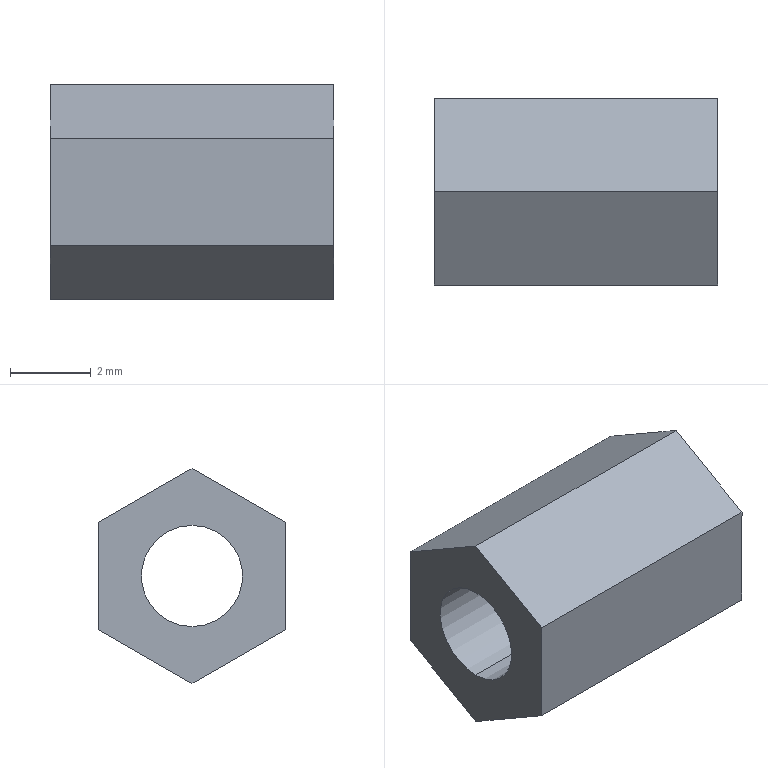Part | SolidWorks | features Extrusion 1, HoleWzd 1 | 1 solid | 10 faces | box 7 x 4.6 x 5.312 mm | volume 93.915 mm3 | plane 8 | cylinder 2 | commonest cylinder face diameters 2.5 x2
STEP:
#1=CARTESIAN_POINT('',(0.,0.,1.25));
#2=VERTEX_POINT('',#1);
#3=CARTESIAN_POINT('',(0.,0.,-1.25));
#4=VERTEX_POINT('',#3);
#5=CARTESIAN_POINT('',(0.,0.,0.));
#6=DIRECTION('',(1.,0.,0.));
#7=DIRECTION('',(0.,0.,-1.));
#8=AXIS2_PLACEMENT_3D('',#5,#6,#7);
#9=CIRCLE('',#8,1.25);
#10=EDGE_CURVE('',#2,#4,#9,.T.);
#11=ORIENTED_EDGE('',*,*,#10,.F.);
#12=CARTESIAN_POINT('',(7.,0.,1.25));
#13=VERTEX_POINT('',#12);
#14=CARTESIAN_POINT('',(7.,0.,1.25));
#15=DIRECTION('',(1.,0.,0.));
#16=VECTOR('',#15,1000.);
#17=LINE('',#14,#16);
#18=EDGE_CURVE('',#2,#13,#17,.T.);
#19=ORIENTED_EDGE('',*,*,#18,.T.);
#20=CARTESIAN_POINT('',(7.,0.,-1.25));
#21=VERTEX_POINT('',#20);
#22=CARTESIAN_POINT('',(7.,0.,0.));
#23=DIRECTION('',(1.,0.,0.));
#24=DIRECTION('',(0.,0.,-1.));
#25=AXIS2_PLACEMENT_3D('',#22,#23,#24);
#26=CIRCLE('',#25,1.25);
#27=EDGE_CURVE('',#13,#21,#26,.T.);
#28=ORIENTED_EDGE('',*,*,#27,.T.);
#29=CARTESIAN_POINT('',(7.,0.,-1.25));
#30=DIRECTION('',(1.,0.,0.));
#31=VECTOR('',#30,1000.);
#32=LINE('',#29,#31);
#33=EDGE_CURVE('',#4,#21,#32,.T.);
#34=ORIENTED_EDGE('',*,*,#33,.F.);
#35=EDGE_LOOP('',(#11,#19,#28,#34));
#36=FACE_OUTER_BOUND('',#35,.T.);
#37=CARTESIAN_POINT('',(7.,0.,0.));
#38=DIRECTION('',(1.,0.,0.));
#39=DIRECTION('',(0.,0.,-1.));
#40=AXIS2_PLACEMENT_3D('',#37,#38,#39);
#41=CYLINDRICAL_SURFACE('',#40,1.25);
#42=ADVANCED_FACE('',(#36),#41,.F.);
#43=CARTESIAN_POINT('',(0.,-2.3,-1.328));
#44=VERTEX_POINT('',#43);
#45=CARTESIAN_POINT('',(0.,0.,-2.656));
#46=VERTEX_POINT('',#45);
#47=CARTESIAN_POINT('',(0.,-2.3,-1.328));
#48=DIRECTION('',(0.,0.866,-0.5));
#49=VECTOR('',#48,1000.);
#50=LINE('',#47,#49);
#51=EDGE_CURVE('',#44,#46,#50,.T.);
#52=ORIENTED_EDGE('',*,*,#51,.T.);
#53=CARTESIAN_POINT('',(7.,0.,-2.656));
#54=VERTEX_POINT('',#53);
#55=CARTESIAN_POINT('',(7.,0.,-2.656));
#56=DIRECTION('',(-1.,0.,0.));
#57=VECTOR('',#56,1000.);
#58=LINE('',#55,#57);
#59=EDGE_CURVE('',#54,#46,#58,.T.);
#60=ORIENTED_EDGE('',*,*,#59,.F.);
#61=CARTESIAN_POINT('',(7.,-2.3,-1.328));
#62=VERTEX_POINT('',#61);
#63=CARTESIAN_POINT('',(7.,-2.3,-1.328));
#64=DIRECTION('',(0.,0.866,-0.5));
#65=VECTOR('',#64,1000.);
#66=LINE('',#63,#65);
#67=EDGE_CURVE('',#62,#54,#66,.T.);
#68=ORIENTED_EDGE('',*,*,#67,.F.);
#69=CARTESIAN_POINT('',(7.,-2.3,-1.328));
#70=DIRECTION('',(-1.,0.,0.));
#71=VECTOR('',#70,1000.);
#72=LINE('',#69,#71);
#73=EDGE_CURVE('',#62,#44,#72,.T.);
#74=ORIENTED_EDGE('',*,*,#73,.T.);
#75=EDGE_LOOP('',(#52,#60,#68,#74));
#76=FACE_OUTER_BOUND('',#75,.T.);
#77=CARTESIAN_POINT('',(7.,-2.3,-1.328));
#78=DIRECTION('',(0.,0.5,0.866));
#79=DIRECTION('',(0.,-0.866,0.5));
#80=AXIS2_PLACEMENT_3D('',#77,#78,#79);
#81=PLANE('',#80);
#82=ADVANCED_FACE('',(#76),#81,.F.);
#83=CARTESIAN_POINT('',(0.,2.3,-1.328));
#84=VERTEX_POINT('',#83);
#85=CARTESIAN_POINT('',(0.,0.,-2.656));
#86=DIRECTION('',(0.,0.866,0.5));
#87=VECTOR('',#86,1000.);
#88=LINE('',#85,#87);
#89=EDGE_CURVE('',#46,#84,#88,.T.);
#90=ORIENTED_EDGE('',*,*,#89,.T.);
#91=CARTESIAN_POINT('',(7.,2.3,-1.328));
#92=VERTEX_POINT('',#91);
#93=CARTESIAN_POINT('',(7.,2.3,-1.328));
#94=DIRECTION('',(-1.,0.,0.));
#95=VECTOR('',#94,1000.);
#96=LINE('',#93,#95);
#97=EDGE_CURVE('',#92,#84,#96,.T.);
#98=ORIENTED_EDGE('',*,*,#97,.F.);
#99=CARTESIAN_POINT('',(7.,0.,-2.656));
#100=DIRECTION('',(0.,0.866,0.5));
#101=VECTOR('',#100,1000.);
#102=LINE('',#99,#101);
#103=EDGE_CURVE('',#54,#92,#102,.T.);
#104=ORIENTED_EDGE('',*,*,#103,.F.);
#105=ORIENTED_EDGE('',*,*,#59,.T.);
#106=EDGE_LOOP('',(#90,#98,#104,#105));
#107=FACE_OUTER_BOUND('',#106,.T.);
#108=CARTESIAN_POINT('',(7.,0.,-2.656));
#109=DIRECTION('',(0.,-0.5,0.866));
#110=DIRECTION('',(0.,-0.866,-0.5));
#111=AXIS2_PLACEMENT_3D('',#108,#109,#110);
#112=PLANE('',#111);
#113=ADVANCED_FACE('',(#107),#112,.F.);
#114=CARTESIAN_POINT('',(0.,2.3,1.328));
#115=VERTEX_POINT('',#114);
#116=CARTESIAN_POINT('',(0.,2.3,-1.328));
#117=DIRECTION('',(0.,0.,1.));
#118=VECTOR('',#117,1000.);
#119=LINE('',#116,#118);
#120=EDGE_CURVE('',#84,#115,#119,.T.);
#121=ORIENTED_EDGE('',*,*,#120,.T.);
#122=CARTESIAN_POINT('',(7.,2.3,1.328));
#123=VERTEX_POINT('',#122);
#124=CARTESIAN_POINT('',(7.,2.3,1.328));
#125=DIRECTION('',(-1.,0.,0.));
#126=VECTOR('',#125,1000.);
#127=LINE('',#124,#126);
#128=EDGE_CURVE('',#123,#115,#127,.T.);
#129=ORIENTED_EDGE('',*,*,#128,.F.);
#130=CARTESIAN_POINT('',(7.,2.3,-1.328));
#131=DIRECTION('',(0.,0.,1.));
#132=VECTOR('',#131,1000.);
#133=LINE('',#130,#132);
#134=EDGE_CURVE('',#92,#123,#133,.T.);
#135=ORIENTED_EDGE('',*,*,#134,.F.);
#136=ORIENTED_EDGE('',*,*,#97,.T.);
#137=EDGE_LOOP('',(#121,#129,#135,#136));
#138=FACE_OUTER_BOUND('',#137,.T.);
#139=CARTESIAN_POINT('',(7.,2.3,-1.328));
#140=DIRECTION('',(0.,-1.,0.));
#141=DIRECTION('',(0.,0.,-1.));
#142=AXIS2_PLACEMENT_3D('',#139,#140,#141);
#143=PLANE('',#142);
#144=ADVANCED_FACE('',(#138),#143,.F.);
#145=CARTESIAN_POINT('',(0.,0.,2.656));
#146=VERTEX_POINT('',#145);
#147=CARTESIAN_POINT('',(0.,2.3,1.328));
#148=DIRECTION('',(0.,-0.866,0.5));
#149=VECTOR('',#148,1000.);
#150=LINE('',#147,#149);
#151=EDGE_CURVE('',#115,#146,#150,.T.);
#152=ORIENTED_EDGE('',*,*,#151,.T.);
#153=CARTESIAN_POINT('',(7.,0.,2.656));
#154=VERTEX_POINT('',#153);
#155=CARTESIAN_POINT('',(7.,0.,2.656));
#156=DIRECTION('',(-1.,0.,0.));
#157=VECTOR('',#156,1000.);
#158=LINE('',#155,#157);
#159=EDGE_CURVE('',#154,#146,#158,.T.);
#160=ORIENTED_EDGE('',*,*,#159,.F.);
#161=CARTESIAN_POINT('',(7.,2.3,1.328));
#162=DIRECTION('',(0.,-0.866,0.5));
#163=VECTOR('',#162,1000.);
#164=LINE('',#161,#163);
#165=EDGE_CURVE('',#123,#154,#164,.T.);
#166=ORIENTED_EDGE('',*,*,#165,.F.);
#167=ORIENTED_EDGE('',*,*,#128,.T.);
#168=EDGE_LOOP('',(#152,#160,#166,#167));
#169=FACE_OUTER_BOUND('',#168,.T.);
#170=CARTESIAN_POINT('',(7.,2.3,1.328));
#171=DIRECTION('',(0.,-0.5,-0.866));
#172=DIRECTION('',(0.,0.866,-0.5));
#173=AXIS2_PLACEMENT_3D('',#170,#171,#172);
#174=PLANE('',#173);
#175=ADVANCED_FACE('',(#169),#174,.F.);
#176=CARTESIAN_POINT('',(0.,-2.3,1.328));
#177=VERTEX_POINT('',#176);
#178=CARTESIAN_POINT('',(0.,0.,2.656));
#179=DIRECTION('',(0.,-0.866,-0.5));
#180=VECTOR('',#179,1000.);
#181=LINE('',#178,#180);
#182=EDGE_CURVE('',#146,#177,#181,.T.);
#183=ORIENTED_EDGE('',*,*,#182,.T.);
#184=CARTESIAN_POINT('',(7.,-2.3,1.328));
#185=VERTEX_POINT('',#184);
#186=CARTESIAN_POINT('',(7.,-2.3,1.328));
#187=DIRECTION('',(-1.,0.,0.));
#188=VECTOR('',#187,1000.);
#189=LINE('',#186,#188);
#190=EDGE_CURVE('',#185,#177,#189,.T.);
#191=ORIENTED_EDGE('',*,*,#190,.F.);
#192=CARTESIAN_POINT('',(7.,0.,2.656));
#193=DIRECTION('',(0.,-0.866,-0.5));
#194=VECTOR('',#193,1000.);
#195=LINE('',#192,#194);
#196=EDGE_CURVE('',#154,#185,#195,.T.);
#197=ORIENTED_EDGE('',*,*,#196,.F.);
#198=ORIENTED_EDGE('',*,*,#159,.T.);
#199=EDGE_LOOP('',(#183,#191,#197,#198));
#200=FACE_OUTER_BOUND('',#199,.T.);
#201=CARTESIAN_POINT('',(7.,0.,2.656));
#202=DIRECTION('',(0.,0.5,-0.866));
#203=DIRECTION('',(0.,0.866,0.5));
#204=AXIS2_PLACEMENT_3D('',#201,#202,#203);
#205=PLANE('',#204);
#206=ADVANCED_FACE('',(#200),#205,.F.);
#207=CARTESIAN_POINT('',(0.,-2.3,1.328));
#208=DIRECTION('',(0.,0.,-1.));
#209=VECTOR('',#208,1000.);
#210=LINE('',#207,#209);
#211=EDGE_CURVE('',#177,#44,#210,.T.);
#212=ORIENTED_EDGE('',*,*,#211,.T.);
#213=ORIENTED_EDGE('',*,*,#73,.F.);
#214=CARTESIAN_POINT('',(7.,-2.3,1.328));
#215=DIRECTION('',(0.,0.,-1.));
#216=VECTOR('',#215,1000.);
#217=LINE('',#214,#216);
#218=EDGE_CURVE('',#185,#62,#217,.T.);
#219=ORIENTED_EDGE('',*,*,#218,.F.);
#220=ORIENTED_EDGE('',*,*,#190,.T.);
#221=EDGE_LOOP('',(#212,#213,#219,#220));
#222=FACE_OUTER_BOUND('',#221,.T.);
#223=CARTESIAN_POINT('',(7.,-2.3,1.328));
#224=DIRECTION('',(0.,1.,0.));
#225=DIRECTION('',(0.,0.,1.));
#226=AXIS2_PLACEMENT_3D('',#223,#224,#225);
#227=PLANE('',#226);
#228=ADVANCED_FACE('',(#222),#227,.F.);
#229=CARTESIAN_POINT('',(7.,0.,0.));
#230=DIRECTION('',(1.,0.,0.));
#231=DIRECTION('',(0.,0.,-1.));
#232=AXIS2_PLACEMENT_3D('',#229,#230,#231);
#233=CIRCLE('',#232,1.25);
#234=EDGE_CURVE('',#21,#13,#233,.T.);
#235=ORIENTED_EDGE('',*,*,#234,.F.);
#236=ORIENTED_EDGE('',*,*,#27,.F.);
#237=EDGE_LOOP('',(#235,#236));
#238=FACE_BOUND('',#237,.T.);
#239=ORIENTED_EDGE('',*,*,#67,.T.);
#240=ORIENTED_EDGE('',*,*,#103,.T.);
#241=ORIENTED_EDGE('',*,*,#134,.T.);
#242=ORIENTED_EDGE('',*,*,#165,.T.);
#243=ORIENTED_EDGE('',*,*,#196,.T.);
#244=ORIENTED_EDGE('',*,*,#218,.T.);
#245=EDGE_LOOP('',(#239,#240,#241,#242,#243,#244));
#246=FACE_OUTER_BOUND('',#245,.T.);
#247=CARTESIAN_POINT('',(7.,0.,0.));
#248=DIRECTION('',(1.,0.,0.));
#249=DIRECTION('',(0.,0.,-1.));
#250=AXIS2_PLACEMENT_3D('',#247,#248,#249);
#251=PLANE('',#250);
#252=ADVANCED_FACE('',(#238,#246),#251,.T.);
#253=CARTESIAN_POINT('',(0.,0.,0.));
#254=DIRECTION('',(1.,0.,0.));
#255=DIRECTION('',(0.,0.,-1.));
#256=AXIS2_PLACEMENT_3D('',#253,#254,#255);
#257=CIRCLE('',#256,1.25);
#258=EDGE_CURVE('',#4,#2,#257,.T.);
#259=ORIENTED_EDGE('',*,*,#258,.T.);
#260=ORIENTED_EDGE('',*,*,#10,.T.);
#261=EDGE_LOOP('',(#259,#260));
#262=FACE_BOUND('',#261,.T.);
#263=ORIENTED_EDGE('',*,*,#51,.F.);
#264=ORIENTED_EDGE('',*,*,#211,.F.);
#265=ORIENTED_EDGE('',*,*,#182,.F.);
#266=ORIENTED_EDGE('',*,*,#151,.F.);
#267=ORIENTED_EDGE('',*,*,#120,.F.);
#268=ORIENTED_EDGE('',*,*,#89,.F.);
#269=EDGE_LOOP('',(#263,#264,#265,#266,#267,#268));
#270=FACE_OUTER_BOUND('',#269,.T.);
#271=CARTESIAN_POINT('',(0.,0.,0.));
#272=DIRECTION('',(1.,0.,0.));
#273=DIRECTION('',(0.,0.,-1.));
#274=AXIS2_PLACEMENT_3D('',#271,#272,#273);
#275=PLANE('',#274);
#276=ADVANCED_FACE('',(#262,#270),#275,.F.);
#277=ORIENTED_EDGE('',*,*,#18,.F.);
#278=ORIENTED_EDGE('',*,*,#258,.F.);
#279=ORIENTED_EDGE('',*,*,#33,.T.);
#280=ORIENTED_EDGE('',*,*,#234,.T.);
#281=EDGE_LOOP('',(#277,#278,#279,#280));
#282=FACE_OUTER_BOUND('',#281,.T.);
#283=CARTESIAN_POINT('',(7.,0.,0.));
#284=DIRECTION('',(1.,0.,0.));
#285=DIRECTION('',(0.,0.,-1.));
#286=AXIS2_PLACEMENT_3D('',#283,#284,#285);
#287=CYLINDRICAL_SURFACE('',#286,1.25);
#288=ADVANCED_FACE('',(#282),#287,.F.);
#289=CLOSED_SHELL('',(#42,#82,#113,#144,#175,#206,#228,#252,#276,#288));
#290=MANIFOLD_SOLID_BREP('',#289);
#291=CARTESIAN_POINT('',(0.,0.,0.));
#292=DIRECTION('',(0.,0.,1.));
#293=DIRECTION('',(1.,0.,0.));
#294=AXIS2_PLACEMENT_3D('',#291,#292,#293);
#295=(LENGTH_UNIT()NAMED_UNIT(*)SI_UNIT(.MILLI.,.METRE.));
#296=UNCERTAINTY_MEASURE_WITH_UNIT(LENGTH_MEASURE(0.00001),#295,'','');
#297=(NAMED_UNIT(*)PLANE_ANGLE_UNIT()SI_UNIT($,.RADIAN.));
#298=(NAMED_UNIT(*)SI_UNIT($,.STERADIAN.)SOLID_ANGLE_UNIT());
#299=(GEOMETRIC_REPRESENTATION_CONTEXT(3)GLOBAL_UNCERTAINTY_ASSIGNED_CONTEXT((#296))GLOBAL_UNIT_ASSIGNED_CONTEXT((#295,#297,#298))REPRESENTATION_CONTEXT('',''));
#300=ADVANCED_BREP_SHAPE_REPRESENTATION('',(#290,#294),#299);